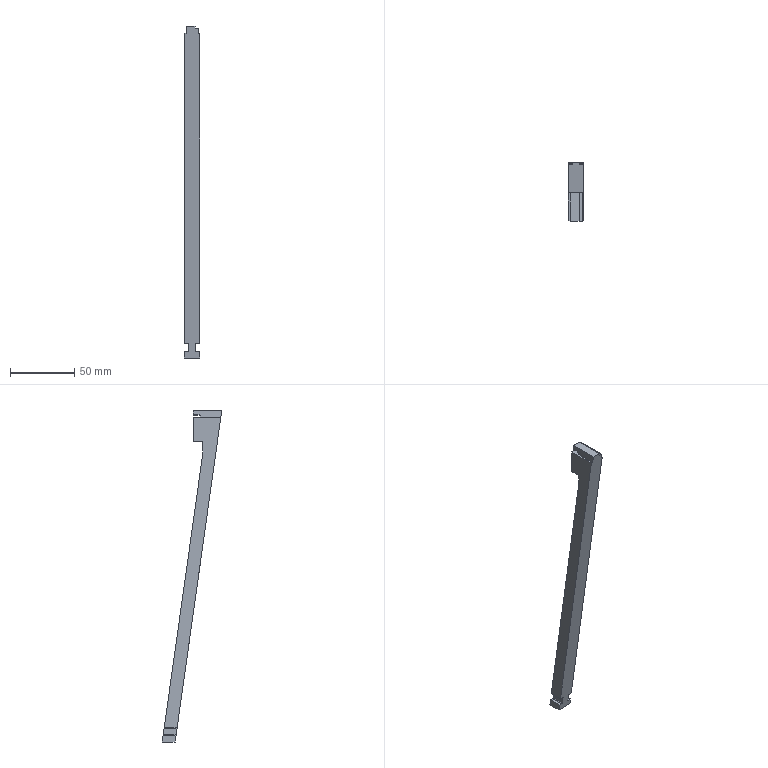Part | Creo | 1 solid | 122 faces | box 12 x 46.477 x 258.85 mm | volume 33483 mm3 | other 67 | plane 48 | cylinder 7 | commonest cylinder face diameters 1 x4 0.92 x1 2 x1 25.168 x1